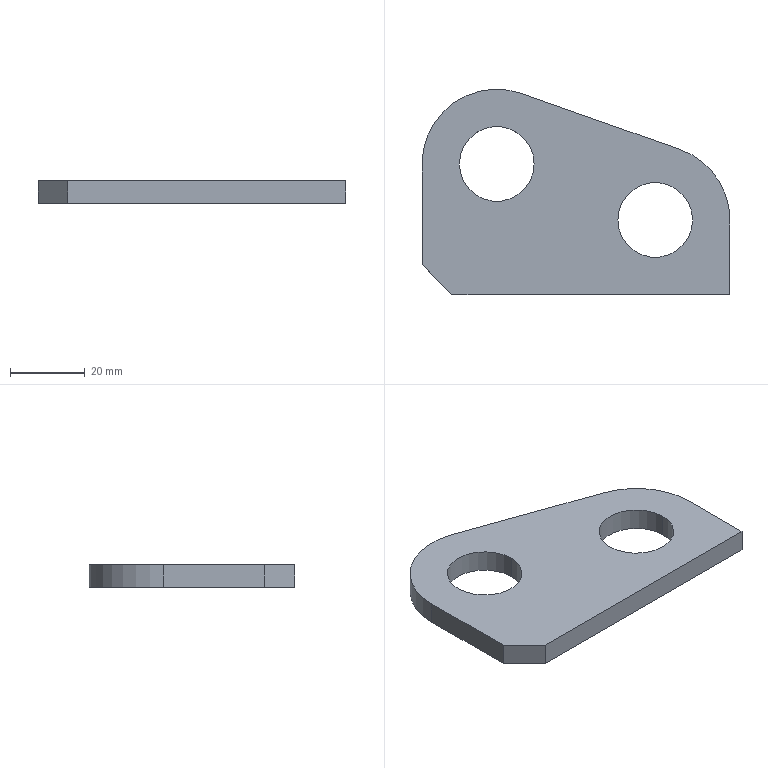Part | SolidWorks | features FlatPattern 1, SMBaseFlange 1, SheetMetal 1 | 1 solid | 13 faces | box 82.426 x 55 x 6 mm | volume 18808 mm3 | plane 7 | cylinder 6 | commonest cylinder face diameters 20 x4 40 x2
STEP:
#1=CARTESIAN_POINT('',(-109.164,-68.574,-6.));
#2=VERTEX_POINT('',#1);
#3=CARTESIAN_POINT('',(-89.164,-68.574,-6.));
#4=VERTEX_POINT('',#3);
#5=CARTESIAN_POINT('',(-99.164,-68.574,-6.));
#6=DIRECTION('',(0.,0.,1.));
#7=DIRECTION('',(1.,0.,0.));
#8=AXIS2_PLACEMENT_3D('',#5,#6,#7);
#9=CIRCLE('',#8,10.);
#10=EDGE_CURVE('',#2,#4,#9,.T.);
#11=ORIENTED_EDGE('',*,*,#10,.F.);
#12=CARTESIAN_POINT('',(-109.164,-68.574,0.));
#13=VERTEX_POINT('',#12);
#14=CARTESIAN_POINT('',(-109.164,-68.574,-6.));
#15=DIRECTION('',(0.,0.,1.));
#16=VECTOR('',#15,1000.);
#17=LINE('',#14,#16);
#18=EDGE_CURVE('',#2,#13,#17,.T.);
#19=ORIENTED_EDGE('',*,*,#18,.T.);
#20=CARTESIAN_POINT('',(-89.164,-68.574,0.));
#21=VERTEX_POINT('',#20);
#22=CARTESIAN_POINT('',(-99.164,-68.574,0.));
#23=DIRECTION('',(0.,0.,1.));
#24=DIRECTION('',(1.,0.,0.));
#25=AXIS2_PLACEMENT_3D('',#22,#23,#24);
#26=CIRCLE('',#25,10.);
#27=EDGE_CURVE('',#13,#21,#26,.T.);
#28=ORIENTED_EDGE('',*,*,#27,.T.);
#29=CARTESIAN_POINT('',(-89.164,-68.574,-6.));
#30=DIRECTION('',(0.,0.,1.));
#31=VECTOR('',#30,1000.);
#32=LINE('',#29,#31);
#33=EDGE_CURVE('',#4,#21,#32,.T.);
#34=ORIENTED_EDGE('',*,*,#33,.F.);
#35=EDGE_LOOP('',(#11,#19,#28,#34));
#36=FACE_OUTER_BOUND('',#35,.T.);
#37=CARTESIAN_POINT('',(-99.164,-68.574,-6.));
#38=DIRECTION('',(0.,0.,1.));
#39=DIRECTION('',(1.,0.,0.));
#40=AXIS2_PLACEMENT_3D('',#37,#38,#39);
#41=CYLINDRICAL_SURFACE('',#40,10.);
#42=ADVANCED_FACE('',(#36),#41,.F.);
#43=CARTESIAN_POINT('',(-151.59,-53.574,-6.));
#44=VERTEX_POINT('',#43);
#45=CARTESIAN_POINT('',(-131.59,-53.574,-6.));
#46=VERTEX_POINT('',#45);
#47=CARTESIAN_POINT('',(-141.59,-53.574,-6.));
#48=DIRECTION('',(0.,0.,1.));
#49=DIRECTION('',(1.,0.,0.));
#50=AXIS2_PLACEMENT_3D('',#47,#48,#49);
#51=CIRCLE('',#50,10.);
#52=EDGE_CURVE('',#44,#46,#51,.T.);
#53=ORIENTED_EDGE('',*,*,#52,.F.);
#54=CARTESIAN_POINT('',(-151.59,-53.574,0.));
#55=VERTEX_POINT('',#54);
#56=CARTESIAN_POINT('',(-151.59,-53.574,-6.));
#57=DIRECTION('',(0.,0.,1.));
#58=VECTOR('',#57,1000.);
#59=LINE('',#56,#58);
#60=EDGE_CURVE('',#44,#55,#59,.T.);
#61=ORIENTED_EDGE('',*,*,#60,.T.);
#62=CARTESIAN_POINT('',(-131.59,-53.574,0.));
#63=VERTEX_POINT('',#62);
#64=CARTESIAN_POINT('',(-141.59,-53.574,0.));
#65=DIRECTION('',(0.,0.,1.));
#66=DIRECTION('',(1.,0.,0.));
#67=AXIS2_PLACEMENT_3D('',#64,#65,#66);
#68=CIRCLE('',#67,10.);
#69=EDGE_CURVE('',#55,#63,#68,.T.);
#70=ORIENTED_EDGE('',*,*,#69,.T.);
#71=CARTESIAN_POINT('',(-131.59,-53.574,-6.));
#72=DIRECTION('',(0.,0.,1.));
#73=VECTOR('',#72,1000.);
#74=LINE('',#71,#73);
#75=EDGE_CURVE('',#46,#63,#74,.T.);
#76=ORIENTED_EDGE('',*,*,#75,.F.);
#77=EDGE_LOOP('',(#53,#61,#70,#76));
#78=FACE_OUTER_BOUND('',#77,.T.);
#79=CARTESIAN_POINT('',(-141.59,-53.574,-6.));
#80=DIRECTION('',(0.,0.,1.));
#81=DIRECTION('',(1.,0.,0.));
#82=AXIS2_PLACEMENT_3D('',#79,#80,#81);
#83=CYLINDRICAL_SURFACE('',#82,10.);
#84=ADVANCED_FACE('',(#78),#83,.F.);
#85=CARTESIAN_POINT('',(-134.924,-34.717,0.));
#86=VERTEX_POINT('',#85);
#87=CARTESIAN_POINT('',(-161.59,-53.574,0.));
#88=VERTEX_POINT('',#87);
#89=CARTESIAN_POINT('',(-141.59,-53.574,0.));
#90=DIRECTION('',(0.,0.,1.));
#91=DIRECTION('',(-1.,0.,0.));
#92=AXIS2_PLACEMENT_3D('',#89,#90,#91);
#93=CIRCLE('',#92,20.);
#94=EDGE_CURVE('',#86,#88,#93,.T.);
#95=ORIENTED_EDGE('',*,*,#94,.F.);
#96=CARTESIAN_POINT('',(-134.924,-34.717,-6.));
#97=VERTEX_POINT('',#96);
#98=CARTESIAN_POINT('',(-134.924,-34.717,-6.));
#99=DIRECTION('',(0.,0.,1.));
#100=VECTOR('',#99,1000.);
#101=LINE('',#98,#100);
#102=EDGE_CURVE('',#97,#86,#101,.T.);
#103=ORIENTED_EDGE('',*,*,#102,.F.);
#104=CARTESIAN_POINT('',(-161.59,-53.574,-6.));
#105=VERTEX_POINT('',#104);
#106=CARTESIAN_POINT('',(-141.59,-53.574,-6.));
#107=DIRECTION('',(0.,0.,1.));
#108=DIRECTION('',(-1.,0.,0.));
#109=AXIS2_PLACEMENT_3D('',#106,#107,#108);
#110=CIRCLE('',#109,20.);
#111=EDGE_CURVE('',#97,#105,#110,.T.);
#112=ORIENTED_EDGE('',*,*,#111,.T.);
#113=CARTESIAN_POINT('',(-161.59,-53.574,-6.));
#114=DIRECTION('',(0.,0.,1.));
#115=VECTOR('',#114,1000.);
#116=LINE('',#113,#115);
#117=EDGE_CURVE('',#105,#88,#116,.T.);
#118=ORIENTED_EDGE('',*,*,#117,.T.);
#119=EDGE_LOOP('',(#95,#103,#112,#118));
#120=FACE_OUTER_BOUND('',#119,.T.);
#121=CARTESIAN_POINT('',(-141.59,-53.574,-6.));
#122=DIRECTION('',(0.,0.,1.));
#123=DIRECTION('',(1.,0.,0.));
#124=AXIS2_PLACEMENT_3D('',#121,#122,#123);
#125=CYLINDRICAL_SURFACE('',#124,20.);
#126=ADVANCED_FACE('',(#120),#125,.T.);
#127=CARTESIAN_POINT('',(-92.497,-49.717,0.));
#128=VERTEX_POINT('',#127);
#129=CARTESIAN_POINT('',(-134.924,-34.717,0.));
#130=DIRECTION('',(-0.9428,0.3333,0.));
#131=VECTOR('',#130,1000.);
#132=LINE('',#129,#131);
#133=EDGE_CURVE('',#128,#86,#132,.T.);
#134=ORIENTED_EDGE('',*,*,#133,.F.);
#135=CARTESIAN_POINT('',(-92.497,-49.717,-6.));
#136=VERTEX_POINT('',#135);
#137=CARTESIAN_POINT('',(-92.497,-49.717,-6.));
#138=DIRECTION('',(0.,0.,1.));
#139=VECTOR('',#138,1000.);
#140=LINE('',#137,#139);
#141=EDGE_CURVE('',#136,#128,#140,.T.);
#142=ORIENTED_EDGE('',*,*,#141,.F.);
#143=CARTESIAN_POINT('',(-134.924,-34.717,-6.));
#144=DIRECTION('',(-0.9428,0.3333,0.));
#145=VECTOR('',#144,1000.);
#146=LINE('',#143,#145);
#147=EDGE_CURVE('',#136,#97,#146,.T.);
#148=ORIENTED_EDGE('',*,*,#147,.T.);
#149=ORIENTED_EDGE('',*,*,#102,.T.);
#150=EDGE_LOOP('',(#134,#142,#148,#149));
#151=FACE_OUTER_BOUND('',#150,.T.);
#152=CARTESIAN_POINT('',(-134.924,-34.717,-6.));
#153=DIRECTION('',(0.3333,0.9428,0.));
#154=DIRECTION('',(-0.9428,0.3333,0.));
#155=AXIS2_PLACEMENT_3D('',#152,#153,#154);
#156=PLANE('',#155);
#157=ADVANCED_FACE('',(#151),#156,.T.);
#158=CARTESIAN_POINT('',(-79.164,-68.574,0.));
#159=VERTEX_POINT('',#158);
#160=CARTESIAN_POINT('',(-99.164,-68.574,0.));
#161=DIRECTION('',(0.,0.,1.));
#162=DIRECTION('',(1.,0.,0.));
#163=AXIS2_PLACEMENT_3D('',#160,#161,#162);
#164=CIRCLE('',#163,20.);
#165=EDGE_CURVE('',#159,#128,#164,.T.);
#166=ORIENTED_EDGE('',*,*,#165,.F.);
#167=CARTESIAN_POINT('',(-79.164,-68.574,-6.));
#168=VERTEX_POINT('',#167);
#169=CARTESIAN_POINT('',(-79.164,-68.574,-6.));
#170=DIRECTION('',(0.,0.,1.));
#171=VECTOR('',#170,1000.);
#172=LINE('',#169,#171);
#173=EDGE_CURVE('',#168,#159,#172,.T.);
#174=ORIENTED_EDGE('',*,*,#173,.F.);
#175=CARTESIAN_POINT('',(-99.164,-68.574,-6.));
#176=DIRECTION('',(0.,0.,1.));
#177=DIRECTION('',(1.,0.,0.));
#178=AXIS2_PLACEMENT_3D('',#175,#176,#177);
#179=CIRCLE('',#178,20.);
#180=EDGE_CURVE('',#168,#136,#179,.T.);
#181=ORIENTED_EDGE('',*,*,#180,.T.);
#182=ORIENTED_EDGE('',*,*,#141,.T.);
#183=EDGE_LOOP('',(#166,#174,#181,#182));
#184=FACE_OUTER_BOUND('',#183,.T.);
#185=CARTESIAN_POINT('',(-99.164,-68.574,-6.));
#186=DIRECTION('',(0.,0.,1.));
#187=DIRECTION('',(1.,0.,0.));
#188=AXIS2_PLACEMENT_3D('',#185,#186,#187);
#189=CYLINDRICAL_SURFACE('',#188,20.);
#190=ADVANCED_FACE('',(#184),#189,.T.);
#191=CARTESIAN_POINT('',(-79.164,-88.574,0.));
#192=VERTEX_POINT('',#191);
#193=CARTESIAN_POINT('',(-79.164,-68.574,0.));
#194=DIRECTION('',(0.,1.,0.));
#195=VECTOR('',#194,1000.);
#196=LINE('',#193,#195);
#197=EDGE_CURVE('',#192,#159,#196,.T.);
#198=ORIENTED_EDGE('',*,*,#197,.F.);
#199=CARTESIAN_POINT('',(-79.164,-88.574,-6.));
#200=VERTEX_POINT('',#199);
#201=CARTESIAN_POINT('',(-79.164,-88.574,-6.));
#202=DIRECTION('',(0.,0.,1.));
#203=VECTOR('',#202,1000.);
#204=LINE('',#201,#203);
#205=EDGE_CURVE('',#200,#192,#204,.T.);
#206=ORIENTED_EDGE('',*,*,#205,.F.);
#207=CARTESIAN_POINT('',(-79.164,-68.574,-6.));
#208=DIRECTION('',(0.,1.,0.));
#209=VECTOR('',#208,1000.);
#210=LINE('',#207,#209);
#211=EDGE_CURVE('',#200,#168,#210,.T.);
#212=ORIENTED_EDGE('',*,*,#211,.T.);
#213=ORIENTED_EDGE('',*,*,#173,.T.);
#214=EDGE_LOOP('',(#198,#206,#212,#213));
#215=FACE_OUTER_BOUND('',#214,.T.);
#216=CARTESIAN_POINT('',(-79.164,-68.574,-6.));
#217=DIRECTION('',(1.,0.,0.));
#218=DIRECTION('',(0.,0.,-1.));
#219=AXIS2_PLACEMENT_3D('',#216,#217,#218);
#220=PLANE('',#219);
#221=ADVANCED_FACE('',(#215),#220,.T.);
#222=CARTESIAN_POINT('',(-153.59,-88.574,0.));
#223=VERTEX_POINT('',#222);
#224=CARTESIAN_POINT('',(-79.164,-88.574,0.));
#225=DIRECTION('',(1.,0.,0.));
#226=VECTOR('',#225,1000.);
#227=LINE('',#224,#226);
#228=EDGE_CURVE('',#223,#192,#227,.T.);
#229=ORIENTED_EDGE('',*,*,#228,.F.);
#230=CARTESIAN_POINT('',(-153.59,-88.574,-6.));
#231=VERTEX_POINT('',#230);
#232=CARTESIAN_POINT('',(-153.59,-88.574,-6.));
#233=DIRECTION('',(0.,0.,1.));
#234=VECTOR('',#233,1000.);
#235=LINE('',#232,#234);
#236=EDGE_CURVE('',#231,#223,#235,.T.);
#237=ORIENTED_EDGE('',*,*,#236,.F.);
#238=CARTESIAN_POINT('',(-79.164,-88.574,-6.));
#239=DIRECTION('',(1.,0.,0.));
#240=VECTOR('',#239,1000.);
#241=LINE('',#238,#240);
#242=EDGE_CURVE('',#231,#200,#241,.T.);
#243=ORIENTED_EDGE('',*,*,#242,.T.);
#244=ORIENTED_EDGE('',*,*,#205,.T.);
#245=EDGE_LOOP('',(#229,#237,#243,#244));
#246=FACE_OUTER_BOUND('',#245,.T.);
#247=CARTESIAN_POINT('',(-79.164,-88.574,-6.));
#248=DIRECTION('',(0.,-1.,0.));
#249=DIRECTION('',(1.,0.,0.));
#250=AXIS2_PLACEMENT_3D('',#247,#248,#249);
#251=PLANE('',#250);
#252=ADVANCED_FACE('',(#246),#251,.T.);
#253=CARTESIAN_POINT('',(-161.59,-80.574,0.));
#254=VERTEX_POINT('',#253);
#255=CARTESIAN_POINT('',(-153.59,-88.574,0.));
#256=DIRECTION('',(0.7071,-0.7071,0.));
#257=VECTOR('',#256,1000.);
#258=LINE('',#255,#257);
#259=EDGE_CURVE('',#254,#223,#258,.T.);
#260=ORIENTED_EDGE('',*,*,#259,.F.);
#261=CARTESIAN_POINT('',(-161.59,-80.574,-6.));
#262=VERTEX_POINT('',#261);
#263=CARTESIAN_POINT('',(-161.59,-80.574,-6.));
#264=DIRECTION('',(0.,0.,1.));
#265=VECTOR('',#264,1000.);
#266=LINE('',#263,#265);
#267=EDGE_CURVE('',#262,#254,#266,.T.);
#268=ORIENTED_EDGE('',*,*,#267,.F.);
#269=CARTESIAN_POINT('',(-153.59,-88.574,-6.));
#270=DIRECTION('',(0.7071,-0.7071,0.));
#271=VECTOR('',#270,1000.);
#272=LINE('',#269,#271);
#273=EDGE_CURVE('',#262,#231,#272,.T.);
#274=ORIENTED_EDGE('',*,*,#273,.T.);
#275=ORIENTED_EDGE('',*,*,#236,.T.);
#276=EDGE_LOOP('',(#260,#268,#274,#275));
#277=FACE_OUTER_BOUND('',#276,.T.);
#278=CARTESIAN_POINT('',(-153.59,-88.574,-6.));
#279=DIRECTION('',(-0.7071,-0.7071,0.));
#280=DIRECTION('',(0.7071,-0.7071,0.));
#281=AXIS2_PLACEMENT_3D('',#278,#279,#280);
#282=PLANE('',#281);
#283=ADVANCED_FACE('',(#277),#282,.T.);
#284=CARTESIAN_POINT('',(-161.59,-80.574,0.));
#285=DIRECTION('',(0.,-1.,0.));
#286=VECTOR('',#285,1000.);
#287=LINE('',#284,#286);
#288=EDGE_CURVE('',#88,#254,#287,.T.);
#289=ORIENTED_EDGE('',*,*,#288,.F.);
#290=ORIENTED_EDGE('',*,*,#117,.F.);
#291=CARTESIAN_POINT('',(-161.59,-80.574,-6.));
#292=DIRECTION('',(0.,-1.,0.));
#293=VECTOR('',#292,1000.);
#294=LINE('',#291,#293);
#295=EDGE_CURVE('',#105,#262,#294,.T.);
#296=ORIENTED_EDGE('',*,*,#295,.T.);
#297=ORIENTED_EDGE('',*,*,#267,.T.);
#298=EDGE_LOOP('',(#289,#290,#296,#297));
#299=FACE_OUTER_BOUND('',#298,.T.);
#300=CARTESIAN_POINT('',(-161.59,-80.574,-6.));
#301=DIRECTION('',(-1.,0.,0.));
#302=DIRECTION('',(0.,-1.,0.));
#303=AXIS2_PLACEMENT_3D('',#300,#301,#302);
#304=PLANE('',#303);
#305=ADVANCED_FACE('',(#299),#304,.T.);
#306=CARTESIAN_POINT('',(-99.164,-68.574,-6.));
#307=DIRECTION('',(0.,0.,1.));
#308=DIRECTION('',(1.,0.,0.));
#309=AXIS2_PLACEMENT_3D('',#306,#307,#308);
#310=CIRCLE('',#309,10.);
#311=EDGE_CURVE('',#4,#2,#310,.T.);
#312=ORIENTED_EDGE('',*,*,#311,.T.);
#313=ORIENTED_EDGE('',*,*,#10,.T.);
#314=EDGE_LOOP('',(#312,#313));
#315=FACE_BOUND('',#314,.T.);
#316=CARTESIAN_POINT('',(-141.59,-53.574,-6.));
#317=DIRECTION('',(0.,0.,1.));
#318=DIRECTION('',(1.,0.,0.));
#319=AXIS2_PLACEMENT_3D('',#316,#317,#318);
#320=CIRCLE('',#319,10.);
#321=EDGE_CURVE('',#46,#44,#320,.T.);
#322=ORIENTED_EDGE('',*,*,#321,.T.);
#323=ORIENTED_EDGE('',*,*,#52,.T.);
#324=EDGE_LOOP('',(#322,#323));
#325=FACE_BOUND('',#324,.T.);
#326=ORIENTED_EDGE('',*,*,#111,.F.);
#327=ORIENTED_EDGE('',*,*,#147,.F.);
#328=ORIENTED_EDGE('',*,*,#180,.F.);
#329=ORIENTED_EDGE('',*,*,#211,.F.);
#330=ORIENTED_EDGE('',*,*,#242,.F.);
#331=ORIENTED_EDGE('',*,*,#273,.F.);
#332=ORIENTED_EDGE('',*,*,#295,.F.);
#333=EDGE_LOOP('',(#326,#327,#328,#329,#330,#331,#332));
#334=FACE_OUTER_BOUND('',#333,.T.);
#335=CARTESIAN_POINT('',(-141.59,-53.574,-6.));
#336=DIRECTION('',(0.,0.,-1.));
#337=DIRECTION('',(-1.,0.,0.));
#338=AXIS2_PLACEMENT_3D('',#335,#336,#337);
#339=PLANE('',#338);
#340=ADVANCED_FACE('',(#315,#325,#334),#339,.T.);
#341=CARTESIAN_POINT('',(-99.164,-68.574,0.));
#342=DIRECTION('',(0.,0.,1.));
#343=DIRECTION('',(1.,0.,0.));
#344=AXIS2_PLACEMENT_3D('',#341,#342,#343);
#345=CIRCLE('',#344,10.);
#346=EDGE_CURVE('',#21,#13,#345,.T.);
#347=ORIENTED_EDGE('',*,*,#346,.F.);
#348=ORIENTED_EDGE('',*,*,#27,.F.);
#349=EDGE_LOOP('',(#347,#348));
#350=FACE_BOUND('',#349,.T.);
#351=CARTESIAN_POINT('',(-141.59,-53.574,0.));
#352=DIRECTION('',(0.,0.,1.));
#353=DIRECTION('',(1.,0.,0.));
#354=AXIS2_PLACEMENT_3D('',#351,#352,#353);
#355=CIRCLE('',#354,10.);
#356=EDGE_CURVE('',#63,#55,#355,.T.);
#357=ORIENTED_EDGE('',*,*,#356,.F.);
#358=ORIENTED_EDGE('',*,*,#69,.F.);
#359=EDGE_LOOP('',(#357,#358));
#360=FACE_BOUND('',#359,.T.);
#361=ORIENTED_EDGE('',*,*,#94,.T.);
#362=ORIENTED_EDGE('',*,*,#288,.T.);
#363=ORIENTED_EDGE('',*,*,#259,.T.);
#364=ORIENTED_EDGE('',*,*,#228,.T.);
#365=ORIENTED_EDGE('',*,*,#197,.T.);
#366=ORIENTED_EDGE('',*,*,#165,.T.);
#367=ORIENTED_EDGE('',*,*,#133,.T.);
#368=EDGE_LOOP('',(#361,#362,#363,#364,#365,#366,#367));
#369=FACE_OUTER_BOUND('',#368,.T.);
#370=CARTESIAN_POINT('',(-141.59,-53.574,0.));
#371=DIRECTION('',(0.,0.,-1.));
#372=DIRECTION('',(-1.,0.,0.));
#373=AXIS2_PLACEMENT_3D('',#370,#371,#372);
#374=PLANE('',#373);
#375=ADVANCED_FACE('',(#350,#360,#369),#374,.F.);
#376=ORIENTED_EDGE('',*,*,#60,.F.);
#377=ORIENTED_EDGE('',*,*,#321,.F.);
#378=ORIENTED_EDGE('',*,*,#75,.T.);
#379=ORIENTED_EDGE('',*,*,#356,.T.);
#380=EDGE_LOOP('',(#376,#377,#378,#379));
#381=FACE_OUTER_BOUND('',#380,.T.);
#382=CARTESIAN_POINT('',(-141.59,-53.574,-6.));
#383=DIRECTION('',(0.,0.,1.));
#384=DIRECTION('',(1.,0.,0.));
#385=AXIS2_PLACEMENT_3D('',#382,#383,#384);
#386=CYLINDRICAL_SURFACE('',#385,10.);
#387=ADVANCED_FACE('',(#381),#386,.F.);
#388=ORIENTED_EDGE('',*,*,#18,.F.);
#389=ORIENTED_EDGE('',*,*,#311,.F.);
#390=ORIENTED_EDGE('',*,*,#33,.T.);
#391=ORIENTED_EDGE('',*,*,#346,.T.);
#392=EDGE_LOOP('',(#388,#389,#390,#391));
#393=FACE_OUTER_BOUND('',#392,.T.);
#394=CARTESIAN_POINT('',(-99.164,-68.574,-6.));
#395=DIRECTION('',(0.,0.,1.));
#396=DIRECTION('',(1.,0.,0.));
#397=AXIS2_PLACEMENT_3D('',#394,#395,#396);
#398=CYLINDRICAL_SURFACE('',#397,10.);
#399=ADVANCED_FACE('',(#393),#398,.F.);
#400=CLOSED_SHELL('',(#42,#84,#126,#157,#190,#221,#252,#283,#305,#340,#375,#387,#399));
#401=MANIFOLD_SOLID_BREP('',#400);
#402=CARTESIAN_POINT('',(0.,0.,0.));
#403=DIRECTION('',(0.,0.,1.));
#404=DIRECTION('',(1.,0.,0.));
#405=AXIS2_PLACEMENT_3D('',#402,#403,#404);
#406=(LENGTH_UNIT()NAMED_UNIT(*)SI_UNIT(.MILLI.,.METRE.));
#407=UNCERTAINTY_MEASURE_WITH_UNIT(LENGTH_MEASURE(0.00001),#406,'','');
#408=(NAMED_UNIT(*)PLANE_ANGLE_UNIT()SI_UNIT($,.RADIAN.));
#409=(NAMED_UNIT(*)SI_UNIT($,.STERADIAN.)SOLID_ANGLE_UNIT());
#410=(GEOMETRIC_REPRESENTATION_CONTEXT(3)GLOBAL_UNCERTAINTY_ASSIGNED_CONTEXT((#407))GLOBAL_UNIT_ASSIGNED_CONTEXT((#406,#408,#409))REPRESENTATION_CONTEXT('',''));
#411=ADVANCED_BREP_SHAPE_REPRESENTATION('',(#401,#405),#410);